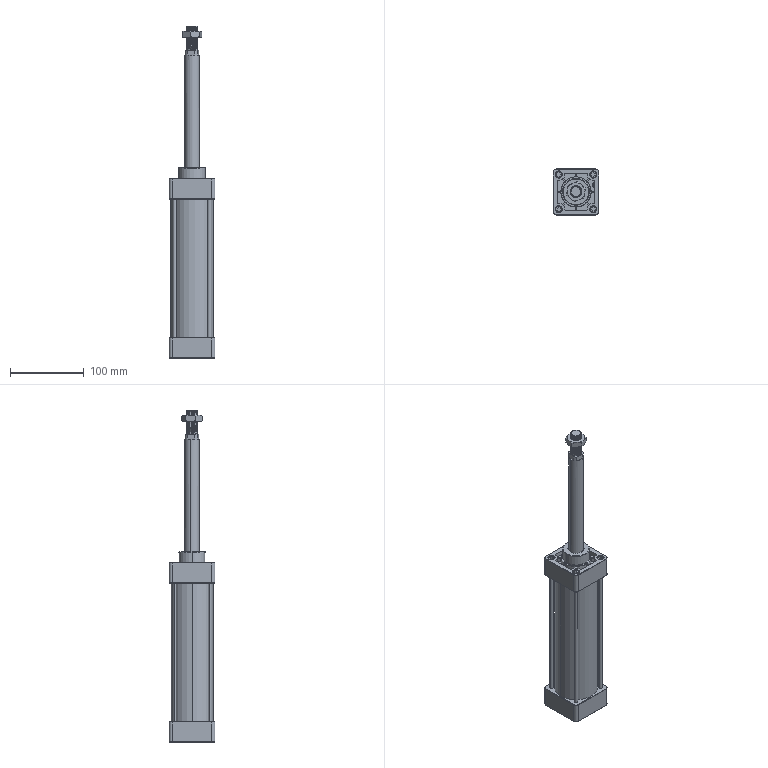Part | SolidWorks | 3 solids | 692 faces | box 62 x 62 x 450 mm | volume 443231 mm3 | plane 319 | cylinder 149 | spline 140 | cone 58 | torus 26 | commonest cylinder face diameters 16 x31 12.301 x30 8.6 x16 9 x16 2 x10 4.5 x8